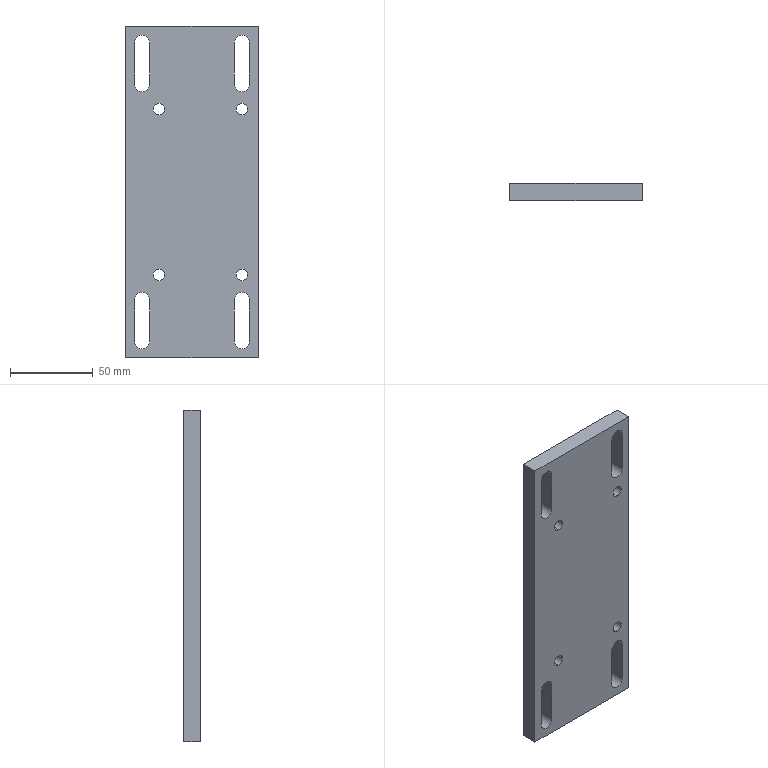Part | STEP file | X77-07007 | 1 solid | 30 faces | box 80 x 10 x 200 mm | volume 147003 mm3 | cylinder 16 | plane 14 | commonest cylinder face diameters 6.8 x8 9 x8
STEP:
#1=CARTESIAN_POINT('',(-304.189,-3.891,153.4));
#2=VERTEX_POINT('',#1);
#3=CARTESIAN_POINT('',(-304.189,-3.891,146.6));
#4=VERTEX_POINT('',#3);
#5=CARTESIAN_POINT('',(-304.189,-3.891,150.));
#6=DIRECTION('',(0.,-1.,0.));
#7=DIRECTION('',(1.,0.,0.));
#8=AXIS2_PLACEMENT_3D('',#5,#6,#7);
#9=CIRCLE('',#8,3.4);
#10=EDGE_CURVE('',#2,#4,#9,.T.);
#11=ORIENTED_EDGE('',*,*,#10,.F.);
#12=CARTESIAN_POINT('',(-304.189,-13.891,153.4));
#13=VERTEX_POINT('',#12);
#14=CARTESIAN_POINT('',(-304.189,-13.891,153.4));
#15=DIRECTION('',(0.,-1.,0.));
#16=VECTOR('',#15,1000.);
#17=LINE('',#14,#16);
#18=EDGE_CURVE('',#2,#13,#17,.T.);
#19=ORIENTED_EDGE('',*,*,#18,.T.);
#20=CARTESIAN_POINT('',(-304.189,-13.891,146.6));
#21=VERTEX_POINT('',#20);
#22=CARTESIAN_POINT('',(-304.189,-13.891,150.));
#23=DIRECTION('',(0.,-1.,0.));
#24=DIRECTION('',(0.,0.,-1.));
#25=AXIS2_PLACEMENT_3D('',#22,#23,#24);
#26=CIRCLE('',#25,3.4);
#27=EDGE_CURVE('',#13,#21,#26,.T.);
#28=ORIENTED_EDGE('',*,*,#27,.T.);
#29=CARTESIAN_POINT('',(-304.189,-13.891,146.6));
#30=DIRECTION('',(0.,-1.,0.));
#31=VECTOR('',#30,1000.);
#32=LINE('',#29,#31);
#33=EDGE_CURVE('',#4,#21,#32,.T.);
#34=ORIENTED_EDGE('',*,*,#33,.F.);
#35=EDGE_LOOP('',(#11,#19,#28,#34));
#36=FACE_OUTER_BOUND('',#35,.T.);
#37=CARTESIAN_POINT('',(-304.189,-13.891,150.));
#38=DIRECTION('',(0.,-1.,0.));
#39=DIRECTION('',(0.,0.,-1.));
#40=AXIS2_PLACEMENT_3D('',#37,#38,#39);
#41=CYLINDRICAL_SURFACE('',#40,3.4);
#42=ADVANCED_FACE('',(#36),#41,.F.);
#43=CARTESIAN_POINT('',(-304.189,-3.891,53.4));
#44=VERTEX_POINT('',#43);
#45=CARTESIAN_POINT('',(-304.189,-3.891,46.6));
#46=VERTEX_POINT('',#45);
#47=CARTESIAN_POINT('',(-304.189,-3.891,50.));
#48=DIRECTION('',(0.,-1.,0.));
#49=DIRECTION('',(1.,0.,0.));
#50=AXIS2_PLACEMENT_3D('',#47,#48,#49);
#51=CIRCLE('',#50,3.4);
#52=EDGE_CURVE('',#44,#46,#51,.T.);
#53=ORIENTED_EDGE('',*,*,#52,.F.);
#54=CARTESIAN_POINT('',(-304.189,-13.891,53.4));
#55=VERTEX_POINT('',#54);
#56=CARTESIAN_POINT('',(-304.189,-13.891,53.4));
#57=DIRECTION('',(0.,-1.,0.));
#58=VECTOR('',#57,1000.);
#59=LINE('',#56,#58);
#60=EDGE_CURVE('',#44,#55,#59,.T.);
#61=ORIENTED_EDGE('',*,*,#60,.T.);
#62=CARTESIAN_POINT('',(-304.189,-13.891,46.6));
#63=VERTEX_POINT('',#62);
#64=CARTESIAN_POINT('',(-304.189,-13.891,50.));
#65=DIRECTION('',(0.,-1.,0.));
#66=DIRECTION('',(0.,0.,-1.));
#67=AXIS2_PLACEMENT_3D('',#64,#65,#66);
#68=CIRCLE('',#67,3.4);
#69=EDGE_CURVE('',#55,#63,#68,.T.);
#70=ORIENTED_EDGE('',*,*,#69,.T.);
#71=CARTESIAN_POINT('',(-304.189,-13.891,46.6));
#72=DIRECTION('',(0.,-1.,0.));
#73=VECTOR('',#72,1000.);
#74=LINE('',#71,#73);
#75=EDGE_CURVE('',#46,#63,#74,.T.);
#76=ORIENTED_EDGE('',*,*,#75,.F.);
#77=EDGE_LOOP('',(#53,#61,#70,#76));
#78=FACE_OUTER_BOUND('',#77,.T.);
#79=CARTESIAN_POINT('',(-304.189,-13.891,50.));
#80=DIRECTION('',(0.,-1.,0.));
#81=DIRECTION('',(0.,0.,-1.));
#82=AXIS2_PLACEMENT_3D('',#79,#80,#81);
#83=CYLINDRICAL_SURFACE('',#82,3.4);
#84=ADVANCED_FACE('',(#78),#83,.F.);
#85=CARTESIAN_POINT('',(-354.189,-3.891,53.4));
#86=VERTEX_POINT('',#85);
#87=CARTESIAN_POINT('',(-354.189,-3.891,46.6));
#88=VERTEX_POINT('',#87);
#89=CARTESIAN_POINT('',(-354.189,-3.891,50.));
#90=DIRECTION('',(0.,-1.,0.));
#91=DIRECTION('',(1.,0.,0.));
#92=AXIS2_PLACEMENT_3D('',#89,#90,#91);
#93=CIRCLE('',#92,3.4);
#94=EDGE_CURVE('',#86,#88,#93,.T.);
#95=ORIENTED_EDGE('',*,*,#94,.F.);
#96=CARTESIAN_POINT('',(-354.189,-13.891,53.4));
#97=VERTEX_POINT('',#96);
#98=CARTESIAN_POINT('',(-354.189,-13.891,53.4));
#99=DIRECTION('',(0.,-1.,0.));
#100=VECTOR('',#99,1000.);
#101=LINE('',#98,#100);
#102=EDGE_CURVE('',#86,#97,#101,.T.);
#103=ORIENTED_EDGE('',*,*,#102,.T.);
#104=CARTESIAN_POINT('',(-354.189,-13.891,46.6));
#105=VERTEX_POINT('',#104);
#106=CARTESIAN_POINT('',(-354.189,-13.891,50.));
#107=DIRECTION('',(0.,-1.,0.));
#108=DIRECTION('',(0.,0.,-1.));
#109=AXIS2_PLACEMENT_3D('',#106,#107,#108);
#110=CIRCLE('',#109,3.4);
#111=EDGE_CURVE('',#97,#105,#110,.T.);
#112=ORIENTED_EDGE('',*,*,#111,.T.);
#113=CARTESIAN_POINT('',(-354.189,-13.891,46.6));
#114=DIRECTION('',(0.,-1.,0.));
#115=VECTOR('',#114,1000.);
#116=LINE('',#113,#115);
#117=EDGE_CURVE('',#88,#105,#116,.T.);
#118=ORIENTED_EDGE('',*,*,#117,.F.);
#119=EDGE_LOOP('',(#95,#103,#112,#118));
#120=FACE_OUTER_BOUND('',#119,.T.);
#121=CARTESIAN_POINT('',(-354.189,-13.891,50.));
#122=DIRECTION('',(0.,-1.,0.));
#123=DIRECTION('',(0.,0.,-1.));
#124=AXIS2_PLACEMENT_3D('',#121,#122,#123);
#125=CYLINDRICAL_SURFACE('',#124,3.4);
#126=ADVANCED_FACE('',(#120),#125,.F.);
#127=CARTESIAN_POINT('',(-354.189,-3.891,153.4));
#128=VERTEX_POINT('',#127);
#129=CARTESIAN_POINT('',(-354.189,-3.891,146.6));
#130=VERTEX_POINT('',#129);
#131=CARTESIAN_POINT('',(-354.189,-3.891,150.));
#132=DIRECTION('',(0.,-1.,0.));
#133=DIRECTION('',(1.,0.,0.));
#134=AXIS2_PLACEMENT_3D('',#131,#132,#133);
#135=CIRCLE('',#134,3.4);
#136=EDGE_CURVE('',#128,#130,#135,.T.);
#137=ORIENTED_EDGE('',*,*,#136,.F.);
#138=CARTESIAN_POINT('',(-354.189,-13.891,153.4));
#139=VERTEX_POINT('',#138);
#140=CARTESIAN_POINT('',(-354.189,-13.891,153.4));
#141=DIRECTION('',(0.,-1.,0.));
#142=VECTOR('',#141,1000.);
#143=LINE('',#140,#142);
#144=EDGE_CURVE('',#128,#139,#143,.T.);
#145=ORIENTED_EDGE('',*,*,#144,.T.);
#146=CARTESIAN_POINT('',(-354.189,-13.891,146.6));
#147=VERTEX_POINT('',#146);
#148=CARTESIAN_POINT('',(-354.189,-13.891,150.));
#149=DIRECTION('',(0.,-1.,0.));
#150=DIRECTION('',(0.,0.,-1.));
#151=AXIS2_PLACEMENT_3D('',#148,#149,#150);
#152=CIRCLE('',#151,3.4);
#153=EDGE_CURVE('',#139,#147,#152,.T.);
#154=ORIENTED_EDGE('',*,*,#153,.T.);
#155=CARTESIAN_POINT('',(-354.189,-13.891,146.6));
#156=DIRECTION('',(0.,-1.,0.));
#157=VECTOR('',#156,1000.);
#158=LINE('',#155,#157);
#159=EDGE_CURVE('',#130,#147,#158,.T.);
#160=ORIENTED_EDGE('',*,*,#159,.F.);
#161=EDGE_LOOP('',(#137,#145,#154,#160));
#162=FACE_OUTER_BOUND('',#161,.T.);
#163=CARTESIAN_POINT('',(-354.189,-13.891,150.));
#164=DIRECTION('',(0.,-1.,0.));
#165=DIRECTION('',(0.,0.,-1.));
#166=AXIS2_PLACEMENT_3D('',#163,#164,#165);
#167=CYLINDRICAL_SURFACE('',#166,3.4);
#168=ADVANCED_FACE('',(#162),#167,.F.);
#169=CARTESIAN_POINT('',(-294.189,-13.891,0.));
#170=VERTEX_POINT('',#169);
#171=CARTESIAN_POINT('',(-294.189,-3.891,0.));
#172=VERTEX_POINT('',#171);
#173=CARTESIAN_POINT('',(-294.189,-13.891,0.));
#174=DIRECTION('',(0.,1.,0.));
#175=VECTOR('',#174,1000.);
#176=LINE('',#173,#175);
#177=EDGE_CURVE('',#170,#172,#176,.T.);
#178=ORIENTED_EDGE('',*,*,#177,.T.);
#179=CARTESIAN_POINT('',(-294.189,-3.891,200.));
#180=VERTEX_POINT('',#179);
#181=CARTESIAN_POINT('',(-294.189,-3.891,200.));
#182=DIRECTION('',(0.,0.,-1.));
#183=VECTOR('',#182,1000.);
#184=LINE('',#181,#183);
#185=EDGE_CURVE('',#180,#172,#184,.T.);
#186=ORIENTED_EDGE('',*,*,#185,.F.);
#187=CARTESIAN_POINT('',(-294.189,-13.891,200.));
#188=VERTEX_POINT('',#187);
#189=CARTESIAN_POINT('',(-294.189,-13.891,200.));
#190=DIRECTION('',(0.,1.,0.));
#191=VECTOR('',#190,1000.);
#192=LINE('',#189,#191);
#193=EDGE_CURVE('',#188,#180,#192,.T.);
#194=ORIENTED_EDGE('',*,*,#193,.F.);
#195=CARTESIAN_POINT('',(-294.189,-13.891,200.));
#196=DIRECTION('',(0.,0.,-1.));
#197=VECTOR('',#196,1000.);
#198=LINE('',#195,#197);
#199=EDGE_CURVE('',#188,#170,#198,.T.);
#200=ORIENTED_EDGE('',*,*,#199,.T.);
#201=EDGE_LOOP('',(#178,#186,#194,#200));
#202=FACE_OUTER_BOUND('',#201,.T.);
#203=CARTESIAN_POINT('',(-294.189,-13.891,200.));
#204=DIRECTION('',(-1.,0.,0.));
#205=DIRECTION('',(0.,0.,1.));
#206=AXIS2_PLACEMENT_3D('',#203,#204,#205);
#207=PLANE('',#206);
#208=ADVANCED_FACE('',(#202),#207,.F.);
#209=CARTESIAN_POINT('',(-368.689,-3.891,35.));
#210=VERTEX_POINT('',#209);
#211=CARTESIAN_POINT('',(-368.689,-3.891,10.));
#212=VERTEX_POINT('',#211);
#213=CARTESIAN_POINT('',(-368.689,-3.891,200.));
#214=DIRECTION('',(0.,0.,-1.));
#215=VECTOR('',#214,1000.);
#216=LINE('',#213,#215);
#217=EDGE_CURVE('',#210,#212,#216,.T.);
#218=ORIENTED_EDGE('',*,*,#217,.T.);
#219=CARTESIAN_POINT('',(-359.689,-3.891,10.));
#220=VERTEX_POINT('',#219);
#221=CARTESIAN_POINT('',(-364.189,-3.891,10.));
#222=DIRECTION('',(0.,-1.,0.));
#223=DIRECTION('',(1.,0.,0.));
#224=AXIS2_PLACEMENT_3D('',#221,#222,#223);
#225=CIRCLE('',#224,4.5);
#226=EDGE_CURVE('',#212,#220,#225,.T.);
#227=ORIENTED_EDGE('',*,*,#226,.T.);
#228=CARTESIAN_POINT('',(-359.689,-3.891,35.));
#229=VERTEX_POINT('',#228);
#230=CARTESIAN_POINT('',(-359.689,-3.891,200.));
#231=DIRECTION('',(0.,0.,1.));
#232=VECTOR('',#231,1000.);
#233=LINE('',#230,#232);
#234=EDGE_CURVE('',#220,#229,#233,.T.);
#235=ORIENTED_EDGE('',*,*,#234,.T.);
#236=CARTESIAN_POINT('',(-364.189,-3.891,35.));
#237=DIRECTION('',(0.,-1.,0.));
#238=DIRECTION('',(1.,0.,0.));
#239=AXIS2_PLACEMENT_3D('',#236,#237,#238);
#240=CIRCLE('',#239,4.5);
#241=EDGE_CURVE('',#229,#210,#240,.T.);
#242=ORIENTED_EDGE('',*,*,#241,.T.);
#243=EDGE_LOOP('',(#218,#227,#235,#242));
#244=FACE_BOUND('',#243,.T.);
#245=CARTESIAN_POINT('',(-359.689,-3.891,165.));
#246=VERTEX_POINT('',#245);
#247=CARTESIAN_POINT('',(-359.689,-3.891,190.));
#248=VERTEX_POINT('',#247);
#249=CARTESIAN_POINT('',(-359.689,-3.891,200.));
#250=DIRECTION('',(0.,0.,1.));
#251=VECTOR('',#250,1000.);
#252=LINE('',#249,#251);
#253=EDGE_CURVE('',#246,#248,#252,.T.);
#254=ORIENTED_EDGE('',*,*,#253,.T.);
#255=CARTESIAN_POINT('',(-368.689,-3.891,190.));
#256=VERTEX_POINT('',#255);
#257=CARTESIAN_POINT('',(-364.189,-3.891,190.));
#258=DIRECTION('',(0.,-1.,0.));
#259=DIRECTION('',(1.,0.,0.));
#260=AXIS2_PLACEMENT_3D('',#257,#258,#259);
#261=CIRCLE('',#260,4.5);
#262=EDGE_CURVE('',#248,#256,#261,.T.);
#263=ORIENTED_EDGE('',*,*,#262,.T.);
#264=CARTESIAN_POINT('',(-368.689,-3.891,165.));
#265=VERTEX_POINT('',#264);
#266=CARTESIAN_POINT('',(-368.689,-3.891,200.));
#267=DIRECTION('',(0.,0.,-1.));
#268=VECTOR('',#267,1000.);
#269=LINE('',#266,#268);
#270=EDGE_CURVE('',#256,#265,#269,.T.);
#271=ORIENTED_EDGE('',*,*,#270,.T.);
#272=CARTESIAN_POINT('',(-364.189,-3.891,165.));
#273=DIRECTION('',(0.,-1.,0.));
#274=DIRECTION('',(1.,0.,0.));
#275=AXIS2_PLACEMENT_3D('',#272,#273,#274);
#276=CIRCLE('',#275,4.5);
#277=EDGE_CURVE('',#265,#246,#276,.T.);
#278=ORIENTED_EDGE('',*,*,#277,.T.);
#279=EDGE_LOOP('',(#254,#263,#271,#278));
#280=FACE_BOUND('',#279,.T.);
#281=CARTESIAN_POINT('',(-308.689,-3.891,35.));
#282=VERTEX_POINT('',#281);
#283=CARTESIAN_POINT('',(-308.689,-3.891,10.));
#284=VERTEX_POINT('',#283);
#285=CARTESIAN_POINT('',(-308.689,-3.891,200.));
#286=DIRECTION('',(0.,0.,-1.));
#287=VECTOR('',#286,1000.);
#288=LINE('',#285,#287);
#289=EDGE_CURVE('',#282,#284,#288,.T.);
#290=ORIENTED_EDGE('',*,*,#289,.T.);
#291=CARTESIAN_POINT('',(-299.689,-3.891,10.));
#292=VERTEX_POINT('',#291);
#293=CARTESIAN_POINT('',(-304.189,-3.891,10.));
#294=DIRECTION('',(0.,-1.,0.));
#295=DIRECTION('',(1.,0.,0.));
#296=AXIS2_PLACEMENT_3D('',#293,#294,#295);
#297=CIRCLE('',#296,4.5);
#298=EDGE_CURVE('',#284,#292,#297,.T.);
#299=ORIENTED_EDGE('',*,*,#298,.T.);
#300=CARTESIAN_POINT('',(-299.689,-3.891,35.));
#301=VERTEX_POINT('',#300);
#302=CARTESIAN_POINT('',(-299.689,-3.891,200.));
#303=DIRECTION('',(0.,0.,1.));
#304=VECTOR('',#303,1000.);
#305=LINE('',#302,#304);
#306=EDGE_CURVE('',#292,#301,#305,.T.);
#307=ORIENTED_EDGE('',*,*,#306,.T.);
#308=CARTESIAN_POINT('',(-304.189,-3.891,35.));
#309=DIRECTION('',(0.,-1.,0.));
#310=DIRECTION('',(1.,0.,0.));
#311=AXIS2_PLACEMENT_3D('',#308,#309,#310);
#312=CIRCLE('',#311,4.5);
#313=EDGE_CURVE('',#301,#282,#312,.T.);
#314=ORIENTED_EDGE('',*,*,#313,.T.);
#315=EDGE_LOOP('',(#290,#299,#307,#314));
#316=FACE_BOUND('',#315,.T.);
#317=CARTESIAN_POINT('',(-299.689,-3.891,165.));
#318=VERTEX_POINT('',#317);
#319=CARTESIAN_POINT('',(-299.689,-3.891,190.));
#320=VERTEX_POINT('',#319);
#321=CARTESIAN_POINT('',(-299.689,-3.891,200.));
#322=DIRECTION('',(0.,0.,1.));
#323=VECTOR('',#322,1000.);
#324=LINE('',#321,#323);
#325=EDGE_CURVE('',#318,#320,#324,.T.);
#326=ORIENTED_EDGE('',*,*,#325,.T.);
#327=CARTESIAN_POINT('',(-308.689,-3.891,190.));
#328=VERTEX_POINT('',#327);
#329=CARTESIAN_POINT('',(-304.189,-3.891,190.));
#330=DIRECTION('',(0.,-1.,0.));
#331=DIRECTION('',(1.,0.,0.));
#332=AXIS2_PLACEMENT_3D('',#329,#330,#331);
#333=CIRCLE('',#332,4.5);
#334=EDGE_CURVE('',#320,#328,#333,.T.);
#335=ORIENTED_EDGE('',*,*,#334,.T.);
#336=CARTESIAN_POINT('',(-308.689,-3.891,165.));
#337=VERTEX_POINT('',#336);
#338=CARTESIAN_POINT('',(-308.689,-3.891,200.));
#339=DIRECTION('',(0.,0.,-1.));
#340=VECTOR('',#339,1000.);
#341=LINE('',#338,#340);
#342=EDGE_CURVE('',#328,#337,#341,.T.);
#343=ORIENTED_EDGE('',*,*,#342,.T.);
#344=CARTESIAN_POINT('',(-304.189,-3.891,165.));
#345=DIRECTION('',(0.,-1.,0.));
#346=DIRECTION('',(1.,0.,0.));
#347=AXIS2_PLACEMENT_3D('',#344,#345,#346);
#348=CIRCLE('',#347,4.5);
#349=EDGE_CURVE('',#337,#318,#348,.T.);
#350=ORIENTED_EDGE('',*,*,#349,.T.);
#351=EDGE_LOOP('',(#326,#335,#343,#350));
#352=FACE_BOUND('',#351,.T.);
#353=CARTESIAN_POINT('',(-304.189,-3.891,150.));
#354=DIRECTION('',(0.,-1.,0.));
#355=DIRECTION('',(1.,0.,0.));
#356=AXIS2_PLACEMENT_3D('',#353,#354,#355);
#357=CIRCLE('',#356,3.4);
#358=EDGE_CURVE('',#4,#2,#357,.T.);
#359=ORIENTED_EDGE('',*,*,#358,.T.);
#360=ORIENTED_EDGE('',*,*,#10,.T.);
#361=EDGE_LOOP('',(#359,#360));
#362=FACE_BOUND('',#361,.T.);
#363=CARTESIAN_POINT('',(-304.189,-3.891,50.));
#364=DIRECTION('',(0.,-1.,0.));
#365=DIRECTION('',(1.,0.,0.));
#366=AXIS2_PLACEMENT_3D('',#363,#364,#365);
#367=CIRCLE('',#366,3.4);
#368=EDGE_CURVE('',#46,#44,#367,.T.);
#369=ORIENTED_EDGE('',*,*,#368,.T.);
#370=ORIENTED_EDGE('',*,*,#52,.T.);
#371=EDGE_LOOP('',(#369,#370));
#372=FACE_BOUND('',#371,.T.);
#373=CARTESIAN_POINT('',(-354.189,-3.891,50.));
#374=DIRECTION('',(0.,-1.,0.));
#375=DIRECTION('',(1.,0.,0.));
#376=AXIS2_PLACEMENT_3D('',#373,#374,#375);
#377=CIRCLE('',#376,3.4);
#378=EDGE_CURVE('',#88,#86,#377,.T.);
#379=ORIENTED_EDGE('',*,*,#378,.T.);
#380=ORIENTED_EDGE('',*,*,#94,.T.);
#381=EDGE_LOOP('',(#379,#380));
#382=FACE_BOUND('',#381,.T.);
#383=CARTESIAN_POINT('',(-354.189,-3.891,150.));
#384=DIRECTION('',(0.,-1.,0.));
#385=DIRECTION('',(1.,0.,0.));
#386=AXIS2_PLACEMENT_3D('',#383,#384,#385);
#387=CIRCLE('',#386,3.4);
#388=EDGE_CURVE('',#130,#128,#387,.T.);
#389=ORIENTED_EDGE('',*,*,#388,.T.);
#390=ORIENTED_EDGE('',*,*,#136,.T.);
#391=EDGE_LOOP('',(#389,#390));
#392=FACE_BOUND('',#391,.T.);
#393=CARTESIAN_POINT('',(-374.189,-3.891,0.));
#394=VERTEX_POINT('',#393);
#395=CARTESIAN_POINT('',(-294.189,-3.891,0.));
#396=DIRECTION('',(-1.,0.,0.));
#397=VECTOR('',#396,1000.);
#398=LINE('',#395,#397);
#399=EDGE_CURVE('',#172,#394,#398,.T.);
#400=ORIENTED_EDGE('',*,*,#399,.T.);
#401=CARTESIAN_POINT('',(-374.189,-3.891,200.));
#402=VERTEX_POINT('',#401);
#403=CARTESIAN_POINT('',(-374.189,-3.891,200.));
#404=DIRECTION('',(0.,0.,-1.));
#405=VECTOR('',#404,1000.);
#406=LINE('',#403,#405);
#407=EDGE_CURVE('',#402,#394,#406,.T.);
#408=ORIENTED_EDGE('',*,*,#407,.F.);
#409=CARTESIAN_POINT('',(-294.189,-3.891,200.));
#410=DIRECTION('',(-1.,0.,0.));
#411=VECTOR('',#410,1000.);
#412=LINE('',#409,#411);
#413=EDGE_CURVE('',#180,#402,#412,.T.);
#414=ORIENTED_EDGE('',*,*,#413,.F.);
#415=ORIENTED_EDGE('',*,*,#185,.T.);
#416=EDGE_LOOP('',(#400,#408,#414,#415));
#417=FACE_OUTER_BOUND('',#416,.T.);
#418=CARTESIAN_POINT('',(-294.189,-3.891,200.));
#419=DIRECTION('',(0.,-1.,0.));
#420=DIRECTION('',(1.,0.,0.));
#421=AXIS2_PLACEMENT_3D('',#418,#419,#420);
#422=PLANE('',#421);
#423=ADVANCED_FACE('',(#244,#280,#316,#352,#362,#372,#382,#392,#417),#422,.F.);
#424=CARTESIAN_POINT('',(-374.189,-13.891,0.));
#425=VERTEX_POINT('',#424);
#426=CARTESIAN_POINT('',(-374.189,-13.891,0.));
#427=DIRECTION('',(0.,-1.,0.));
#428=VECTOR('',#427,1000.);
#429=LINE('',#426,#428);
#430=EDGE_CURVE('',#394,#425,#429,.T.);
#431=ORIENTED_EDGE('',*,*,#430,.T.);
#432=CARTESIAN_POINT('',(-374.189,-13.891,200.));
#433=VERTEX_POINT('',#432);
#434=CARTESIAN_POINT('',(-374.189,-13.891,200.));
#435=DIRECTION('',(0.,0.,-1.));
#436=VECTOR('',#435,1000.);
#437=LINE('',#434,#436);
#438=EDGE_CURVE('',#433,#425,#437,.T.);
#439=ORIENTED_EDGE('',*,*,#438,.F.);
#440=CARTESIAN_POINT('',(-374.189,-13.891,200.));
#441=DIRECTION('',(0.,-1.,0.));
#442=VECTOR('',#441,1000.);
#443=LINE('',#440,#442);
#444=EDGE_CURVE('',#402,#433,#443,.T.);
#445=ORIENTED_EDGE('',*,*,#444,.F.);
#446=ORIENTED_EDGE('',*,*,#407,.T.);
#447=EDGE_LOOP('',(#431,#439,#445,#446));
#448=FACE_OUTER_BOUND('',#447,.T.);
#449=CARTESIAN_POINT('',(-374.189,-13.891,200.));
#450=DIRECTION('',(1.,0.,0.));
#451=DIRECTION('',(0.,0.,-1.));
#452=AXIS2_PLACEMENT_3D('',#449,#450,#451);
#453=PLANE('',#452);
#454=ADVANCED_FACE('',(#448),#453,.F.);
#455=CARTESIAN_POINT('',(-359.689,-13.891,10.));
#456=VERTEX_POINT('',#455);
#457=CARTESIAN_POINT('',(-359.689,-13.891,35.));
#458=VERTEX_POINT('',#457);
#459=CARTESIAN_POINT('',(-359.689,-13.891,10.));
#460=DIRECTION('',(0.,0.,1.));
#461=VECTOR('',#460,1000.);
#462=LINE('',#459,#461);
#463=EDGE_CURVE('',#456,#458,#462,.T.);
#464=ORIENTED_EDGE('',*,*,#463,.F.);
#465=CARTESIAN_POINT('',(-368.689,-13.891,10.));
#466=VERTEX_POINT('',#465);
#467=CARTESIAN_POINT('',(-364.189,-13.891,10.));
#468=DIRECTION('',(0.,-1.,0.));
#469=DIRECTION('',(1.,0.,0.));
#470=AXIS2_PLACEMENT_3D('',#467,#468,#469);
#471=CIRCLE('',#470,4.5);
#472=EDGE_CURVE('',#466,#456,#471,.T.);
#473=ORIENTED_EDGE('',*,*,#472,.F.);
#474=CARTESIAN_POINT('',(-368.689,-13.891,35.));
#475=VERTEX_POINT('',#474);
#476=CARTESIAN_POINT('',(-368.689,-13.891,10.));
#477=DIRECTION('',(0.,0.,-1.));
#478=VECTOR('',#477,1000.);
#479=LINE('',#476,#478);
#480=EDGE_CURVE('',#475,#466,#479,.T.);
#481=ORIENTED_EDGE('',*,*,#480,.F.);
#482=CARTESIAN_POINT('',(-364.189,-13.891,35.));
#483=DIRECTION('',(0.,-1.,0.));
#484=DIRECTION('',(1.,0.,0.));
#485=AXIS2_PLACEMENT_3D('',#482,#483,#484);
#486=CIRCLE('',#485,4.5);
#487=EDGE_CURVE('',#458,#475,#486,.T.);
#488=ORIENTED_EDGE('',*,*,#487,.F.);
#489=EDGE_LOOP('',(#464,#473,#481,#488));
#490=FACE_BOUND('',#489,.T.);
#491=CARTESIAN_POINT('',(-368.689,-13.891,190.));
#492=VERTEX_POINT('',#491);
#493=CARTESIAN_POINT('',(-368.689,-13.891,165.));
#494=VERTEX_POINT('',#493);
#495=CARTESIAN_POINT('',(-368.689,-13.891,190.));
#496=DIRECTION('',(0.,0.,-1.));
#497=VECTOR('',#496,1000.);
#498=LINE('',#495,#497);
#499=EDGE_CURVE('',#492,#494,#498,.T.);
#500=ORIENTED_EDGE('',*,*,#499,.F.);
#501=CARTESIAN_POINT('',(-359.689,-13.891,190.));
#502=VERTEX_POINT('',#501);
#503=CARTESIAN_POINT('',(-364.189,-13.891,190.));
#504=DIRECTION('',(0.,-1.,0.));
#505=DIRECTION('',(-1.,0.,0.));
#506=AXIS2_PLACEMENT_3D('',#503,#504,#505);
#507=CIRCLE('',#506,4.5);
#508=EDGE_CURVE('',#502,#492,#507,.T.);
#509=ORIENTED_EDGE('',*,*,#508,.F.);
#510=CARTESIAN_POINT('',(-359.689,-13.891,165.));
#511=VERTEX_POINT('',#510);
#512=CARTESIAN_POINT('',(-359.689,-13.891,190.));
#513=DIRECTION('',(0.,0.,1.));
#514=VECTOR('',#513,1000.);
#515=LINE('',#512,#514);
#516=EDGE_CURVE('',#511,#502,#515,.T.);
#517=ORIENTED_EDGE('',*,*,#516,.F.);
#518=CARTESIAN_POINT('',(-364.189,-13.891,165.));
#519=DIRECTION('',(0.,-1.,0.));
#520=DIRECTION('',(-1.,0.,0.));
#521=AXIS2_PLACEMENT_3D('',#518,#519,#520);
#522=CIRCLE('',#521,4.5);
#523=EDGE_CURVE('',#494,#511,#522,.T.);
#524=ORIENTED_EDGE('',*,*,#523,.F.);
#525=EDGE_LOOP('',(#500,#509,#517,#524));
#526=FACE_BOUND('',#525,.T.);
#527=CARTESIAN_POINT('',(-299.689,-13.891,10.));
#528=VERTEX_POINT('',#527);
#529=CARTESIAN_POINT('',(-299.689,-13.891,35.));
#530=VERTEX_POINT('',#529);
#531=CARTESIAN_POINT('',(-299.689,-13.891,10.));
#532=DIRECTION('',(0.,0.,1.));
#533=VECTOR('',#532,1000.);
#534=LINE('',#531,#533);
#535=EDGE_CURVE('',#528,#530,#534,.T.);
#536=ORIENTED_EDGE('',*,*,#535,.F.);
#537=CARTESIAN_POINT('',(-308.689,-13.891,10.));
#538=VERTEX_POINT('',#537);
#539=CARTESIAN_POINT('',(-304.189,-13.891,10.));
#540=DIRECTION('',(0.,-1.,0.));
#541=DIRECTION('',(-1.,0.,0.));
#542=AXIS2_PLACEMENT_3D('',#539,#540,#541);
#543=CIRCLE('',#542,4.5);
#544=EDGE_CURVE('',#538,#528,#543,.T.);
#545=ORIENTED_EDGE('',*,*,#544,.F.);
#546=CARTESIAN_POINT('',(-308.689,-13.891,35.));
#547=VERTEX_POINT('',#546);
#548=CARTESIAN_POINT('',(-308.689,-13.891,10.));
#549=DIRECTION('',(0.,0.,-1.));
#550=VECTOR('',#549,1000.);
#551=LINE('',#548,#550);
#552=EDGE_CURVE('',#547,#538,#551,.T.);
#553=ORIENTED_EDGE('',*,*,#552,.F.);
#554=CARTESIAN_POINT('',(-304.189,-13.891,35.));
#555=DIRECTION('',(0.,-1.,0.));
#556=DIRECTION('',(-1.,0.,0.));
#557=AXIS2_PLACEMENT_3D('',#554,#555,#556);
#558=CIRCLE('',#557,4.5);
#559=EDGE_CURVE('',#530,#547,#558,.T.);
#560=ORIENTED_EDGE('',*,*,#559,.F.);
#561=EDGE_LOOP('',(#536,#545,#553,#560));
#562=FACE_BOUND('',#561,.T.);
#563=CARTESIAN_POINT('',(-308.689,-13.891,190.));
#564=VERTEX_POINT('',#563);
#565=CARTESIAN_POINT('',(-308.689,-13.891,165.));
#566=VERTEX_POINT('',#565);
#567=CARTESIAN_POINT('',(-308.689,-13.891,190.));
#568=DIRECTION('',(0.,0.,-1.));
#569=VECTOR('',#568,1000.);
#570=LINE('',#567,#569);
#571=EDGE_CURVE('',#564,#566,#570,.T.);
#572=ORIENTED_EDGE('',*,*,#571,.F.);
#573=CARTESIAN_POINT('',(-299.689,-13.891,190.));
#574=VERTEX_POINT('',#573);
#575=CARTESIAN_POINT('',(-304.189,-13.891,190.));
#576=DIRECTION('',(0.,-1.,0.));
#577=DIRECTION('',(1.,0.,0.));
#578=AXIS2_PLACEMENT_3D('',#575,#576,#577);
#579=CIRCLE('',#578,4.5);
#580=EDGE_CURVE('',#574,#564,#579,.T.);
#581=ORIENTED_EDGE('',*,*,#580,.F.);
#582=CARTESIAN_POINT('',(-299.689,-13.891,165.));
#583=VERTEX_POINT('',#582);
#584=CARTESIAN_POINT('',(-299.689,-13.891,190.));
#585=DIRECTION('',(0.,0.,1.));
#586=VECTOR('',#585,1000.);
#587=LINE('',#584,#586);
#588=EDGE_CURVE('',#583,#574,#587,.T.);
#589=ORIENTED_EDGE('',*,*,#588,.F.);
#590=CARTESIAN_POINT('',(-304.189,-13.891,165.));
#591=DIRECTION('',(0.,-1.,0.));
#592=DIRECTION('',(1.,0.,0.));
#593=AXIS2_PLACEMENT_3D('',#590,#591,#592);
#594=CIRCLE('',#593,4.5);
#595=EDGE_CURVE('',#566,#583,#594,.T.);
#596=ORIENTED_EDGE('',*,*,#595,.F.);
#597=EDGE_LOOP('',(#572,#581,#589,#596));
#598=FACE_BOUND('',#597,.T.);
#599=CARTESIAN_POINT('',(-304.189,-13.891,150.));
#600=DIRECTION('',(0.,-1.,0.));
#601=DIRECTION('',(0.,0.,-1.));
#602=AXIS2_PLACEMENT_3D('',#599,#600,#601);
#603=CIRCLE('',#602,3.4);
#604=EDGE_CURVE('',#21,#13,#603,.T.);
#605=ORIENTED_EDGE('',*,*,#604,.F.);
#606=ORIENTED_EDGE('',*,*,#27,.F.);
#607=EDGE_LOOP('',(#605,#606));
#608=FACE_BOUND('',#607,.T.);
#609=CARTESIAN_POINT('',(-304.189,-13.891,50.));
#610=DIRECTION('',(0.,-1.,0.));
#611=DIRECTION('',(0.,0.,-1.));
#612=AXIS2_PLACEMENT_3D('',#609,#610,#611);
#613=CIRCLE('',#612,3.4);
#614=EDGE_CURVE('',#63,#55,#613,.T.);
#615=ORIENTED_EDGE('',*,*,#614,.F.);
#616=ORIENTED_EDGE('',*,*,#69,.F.);
#617=EDGE_LOOP('',(#615,#616));
#618=FACE_BOUND('',#617,.T.);
#619=CARTESIAN_POINT('',(-354.189,-13.891,50.));
#620=DIRECTION('',(0.,-1.,0.));
#621=DIRECTION('',(0.,0.,-1.));
#622=AXIS2_PLACEMENT_3D('',#619,#620,#621);
#623=CIRCLE('',#622,3.4);
#624=EDGE_CURVE('',#105,#97,#623,.T.);
#625=ORIENTED_EDGE('',*,*,#624,.F.);
#626=ORIENTED_EDGE('',*,*,#111,.F.);
#627=EDGE_LOOP('',(#625,#626));
#628=FACE_BOUND('',#627,.T.);
#629=CARTESIAN_POINT('',(-354.189,-13.891,150.));
#630=DIRECTION('',(0.,-1.,0.));
#631=DIRECTION('',(0.,0.,-1.));
#632=AXIS2_PLACEMENT_3D('',#629,#630,#631);
#633=CIRCLE('',#632,3.4);
#634=EDGE_CURVE('',#147,#139,#633,.T.);
#635=ORIENTED_EDGE('',*,*,#634,.F.);
#636=ORIENTED_EDGE('',*,*,#153,.F.);
#637=EDGE_LOOP('',(#635,#636));
#638=FACE_BOUND('',#637,.T.);
#639=CARTESIAN_POINT('',(-294.189,-13.891,0.));
#640=DIRECTION('',(1.,0.,0.));
#641=VECTOR('',#640,1000.);
#642=LINE('',#639,#641);
#643=EDGE_CURVE('',#425,#170,#642,.T.);
#644=ORIENTED_EDGE('',*,*,#643,.T.);
#645=ORIENTED_EDGE('',*,*,#199,.F.);
#646=CARTESIAN_POINT('',(-294.189,-13.891,200.));
#647=DIRECTION('',(1.,0.,0.));
#648=VECTOR('',#647,1000.);
#649=LINE('',#646,#648);
#650=EDGE_CURVE('',#433,#188,#649,.T.);
#651=ORIENTED_EDGE('',*,*,#650,.F.);
#652=ORIENTED_EDGE('',*,*,#438,.T.);
#653=EDGE_LOOP('',(#644,#645,#651,#652));
#654=FACE_OUTER_BOUND('',#653,.T.);
#655=CARTESIAN_POINT('',(-294.189,-13.891,200.));
#656=DIRECTION('',(0.,1.,0.));
#657=DIRECTION('',(-1.,0.,0.));
#658=AXIS2_PLACEMENT_3D('',#655,#656,#657);
#659=PLANE('',#658);
#660=ADVANCED_FACE('',(#490,#526,#562,#598,#608,#618,#628,#638,#654),#659,.F.);
#661=ORIENTED_EDGE('',*,*,#193,.T.);
#662=ORIENTED_EDGE('',*,*,#413,.T.);
#663=ORIENTED_EDGE('',*,*,#444,.T.);
#664=ORIENTED_EDGE('',*,*,#650,.T.);
#665=EDGE_LOOP('',(#661,#662,#663,#664));
#666=FACE_OUTER_BOUND('',#665,.T.);
#667=CARTESIAN_POINT('',(-294.189,-3.891,200.));
#668=DIRECTION('',(0.,0.,1.));
#669=DIRECTION('',(1.,0.,0.));
#670=AXIS2_PLACEMENT_3D('',#667,#668,#669);
#671=PLANE('',#670);
#672=ADVANCED_FACE('',(#666),#671,.T.);
#673=ORIENTED_EDGE('',*,*,#177,.F.);
#674=ORIENTED_EDGE('',*,*,#643,.F.);
#675=ORIENTED_EDGE('',*,*,#430,.F.);
#676=ORIENTED_EDGE('',*,*,#399,.F.);
#677=EDGE_LOOP('',(#673,#674,#675,#676));
#678=FACE_OUTER_BOUND('',#677,.T.);
#679=CARTESIAN_POINT('',(-294.189,-3.891,0.));
#680=DIRECTION('',(0.,0.,1.));
#681=DIRECTION('',(1.,0.,0.));
#682=AXIS2_PLACEMENT_3D('',#679,#680,#681);
#683=PLANE('',#682);
#684=ADVANCED_FACE('',(#678),#683,.F.);
#685=ORIENTED_EDGE('',*,*,#144,.F.);
#686=ORIENTED_EDGE('',*,*,#388,.F.);
#687=ORIENTED_EDGE('',*,*,#159,.T.);
#688=ORIENTED_EDGE('',*,*,#634,.T.);
#689=EDGE_LOOP('',(#685,#686,#687,#688));
#690=FACE_OUTER_BOUND('',#689,.T.);
#691=CARTESIAN_POINT('',(-354.189,-13.891,150.));
#692=DIRECTION('',(0.,-1.,0.));
#693=DIRECTION('',(0.,0.,-1.));
#694=AXIS2_PLACEMENT_3D('',#691,#692,#693);
#695=CYLINDRICAL_SURFACE('',#694,3.4);
#696=ADVANCED_FACE('',(#690),#695,.F.);
#697=ORIENTED_EDGE('',*,*,#102,.F.);
#698=ORIENTED_EDGE('',*,*,#378,.F.);
#699=ORIENTED_EDGE('',*,*,#117,.T.);
#700=ORIENTED_EDGE('',*,*,#624,.T.);
#701=EDGE_LOOP('',(#697,#698,#699,#700));
#702=FACE_OUTER_BOUND('',#701,.T.);
#703=CARTESIAN_POINT('',(-354.189,-13.891,50.));
#704=DIRECTION('',(0.,-1.,0.));
#705=DIRECTION('',(0.,0.,-1.));
#706=AXIS2_PLACEMENT_3D('',#703,#704,#705);
#707=CYLINDRICAL_SURFACE('',#706,3.4);
#708=ADVANCED_FACE('',(#702),#707,.F.);
#709=ORIENTED_EDGE('',*,*,#60,.F.);
#710=ORIENTED_EDGE('',*,*,#368,.F.);
#711=ORIENTED_EDGE('',*,*,#75,.T.);
#712=ORIENTED_EDGE('',*,*,#614,.T.);
#713=EDGE_LOOP('',(#709,#710,#711,#712));
#714=FACE_OUTER_BOUND('',#713,.T.);
#715=CARTESIAN_POINT('',(-304.189,-13.891,50.));
#716=DIRECTION('',(0.,-1.,0.));
#717=DIRECTION('',(0.,0.,-1.));
#718=AXIS2_PLACEMENT_3D('',#715,#716,#717);
#719=CYLINDRICAL_SURFACE('',#718,3.4);
#720=ADVANCED_FACE('',(#714),#719,.F.);
#721=ORIENTED_EDGE('',*,*,#18,.F.);
#722=ORIENTED_EDGE('',*,*,#358,.F.);
#723=ORIENTED_EDGE('',*,*,#33,.T.);
#724=ORIENTED_EDGE('',*,*,#604,.T.);
#725=EDGE_LOOP('',(#721,#722,#723,#724));
#726=FACE_OUTER_BOUND('',#725,.T.);
#727=CARTESIAN_POINT('',(-304.189,-13.891,150.));
#728=DIRECTION('',(0.,-1.,0.));
#729=DIRECTION('',(0.,0.,-1.));
#730=AXIS2_PLACEMENT_3D('',#727,#728,#729);
#731=CYLINDRICAL_SURFACE('',#730,3.4);
#732=ADVANCED_FACE('',(#726),#731,.F.);
#733=CARTESIAN_POINT('',(-299.689,286.109,190.));
#734=DIRECTION('',(0.,-1.,0.));
#735=VECTOR('',#734,1000.);
#736=LINE('',#733,#735);
#737=EDGE_CURVE('',#320,#574,#736,.T.);
#738=ORIENTED_EDGE('',*,*,#737,.T.);
#739=ORIENTED_EDGE('',*,*,#580,.T.);
#740=CARTESIAN_POINT('',(-308.689,286.109,190.));
#741=DIRECTION('',(0.,-1.,0.));
#742=VECTOR('',#741,1000.);
#743=LINE('',#740,#742);
#744=EDGE_CURVE('',#328,#564,#743,.T.);
#745=ORIENTED_EDGE('',*,*,#744,.F.);
#746=ORIENTED_EDGE('',*,*,#334,.F.);
#747=EDGE_LOOP('',(#738,#739,#745,#746));
#748=FACE_OUTER_BOUND('',#747,.T.);
#749=CARTESIAN_POINT('',(-304.189,286.109,190.));
#750=DIRECTION('',(0.,-1.,0.));
#751=DIRECTION('',(1.,0.,0.));
#752=AXIS2_PLACEMENT_3D('',#749,#750,#751);
#753=CYLINDRICAL_SURFACE('',#752,4.5);
#754=ADVANCED_FACE('',(#748),#753,.F.);
#755=CARTESIAN_POINT('',(-299.689,286.109,165.));
#756=DIRECTION('',(0.,-1.,0.));
#757=VECTOR('',#756,1000.);
#758=LINE('',#755,#757);
#759=EDGE_CURVE('',#318,#583,#758,.T.);
#760=ORIENTED_EDGE('',*,*,#759,.T.);
#761=ORIENTED_EDGE('',*,*,#588,.T.);
#762=ORIENTED_EDGE('',*,*,#737,.F.);
#763=ORIENTED_EDGE('',*,*,#325,.F.);
#764=EDGE_LOOP('',(#760,#761,#762,#763));
#765=FACE_OUTER_BOUND('',#764,.T.);
#766=CARTESIAN_POINT('',(-299.689,286.109,190.));
#767=DIRECTION('',(1.,0.,0.));
#768=DIRECTION('',(0.,1.,0.));
#769=AXIS2_PLACEMENT_3D('',#766,#767,#768);
#770=PLANE('',#769);
#771=ADVANCED_FACE('',(#765),#770,.F.);
#772=CARTESIAN_POINT('',(-308.689,286.109,165.));
#773=DIRECTION('',(0.,-1.,0.));
#774=VECTOR('',#773,1000.);
#775=LINE('',#772,#774);
#776=EDGE_CURVE('',#337,#566,#775,.T.);
#777=ORIENTED_EDGE('',*,*,#776,.T.);
#778=ORIENTED_EDGE('',*,*,#595,.T.);
#779=ORIENTED_EDGE('',*,*,#759,.F.);
#780=ORIENTED_EDGE('',*,*,#349,.F.);
#781=EDGE_LOOP('',(#777,#778,#779,#780));
#782=FACE_OUTER_BOUND('',#781,.T.);
#783=CARTESIAN_POINT('',(-304.189,286.109,165.));
#784=DIRECTION('',(0.,-1.,0.));
#785=DIRECTION('',(1.,0.,0.));
#786=AXIS2_PLACEMENT_3D('',#783,#784,#785);
#787=CYLINDRICAL_SURFACE('',#786,4.5);
#788=ADVANCED_FACE('',(#782),#787,.F.);
#789=ORIENTED_EDGE('',*,*,#744,.T.);
#790=ORIENTED_EDGE('',*,*,#571,.T.);
#791=ORIENTED_EDGE('',*,*,#776,.F.);
#792=ORIENTED_EDGE('',*,*,#342,.F.);
#793=EDGE_LOOP('',(#789,#790,#791,#792));
#794=FACE_OUTER_BOUND('',#793,.T.);
#795=CARTESIAN_POINT('',(-308.689,286.109,190.));
#796=DIRECTION('',(-1.,0.,0.));
#797=DIRECTION('',(0.,-1.,0.));
#798=AXIS2_PLACEMENT_3D('',#795,#796,#797);
#799=PLANE('',#798);
#800=ADVANCED_FACE('',(#794),#799,.F.);
#801=CARTESIAN_POINT('',(-308.689,286.109,10.));
#802=DIRECTION('',(0.,-1.,0.));
#803=VECTOR('',#802,1000.);
#804=LINE('',#801,#803);
#805=EDGE_CURVE('',#284,#538,#804,.T.);
#806=ORIENTED_EDGE('',*,*,#805,.T.);
#807=ORIENTED_EDGE('',*,*,#544,.T.);
#808=CARTESIAN_POINT('',(-299.689,286.109,10.));
#809=DIRECTION('',(0.,-1.,0.));
#810=VECTOR('',#809,1000.);
#811=LINE('',#808,#810);
#812=EDGE_CURVE('',#292,#528,#811,.T.);
#813=ORIENTED_EDGE('',*,*,#812,.F.);
#814=ORIENTED_EDGE('',*,*,#298,.F.);
#815=EDGE_LOOP('',(#806,#807,#813,#814));
#816=FACE_OUTER_BOUND('',#815,.T.);
#817=CARTESIAN_POINT('',(-304.189,286.109,10.));
#818=DIRECTION('',(0.,-1.,0.));
#819=DIRECTION('',(1.,0.,0.));
#820=AXIS2_PLACEMENT_3D('',#817,#818,#819);
#821=CYLINDRICAL_SURFACE('',#820,4.5);
#822=ADVANCED_FACE('',(#816),#821,.F.);
#823=CARTESIAN_POINT('',(-308.689,286.109,35.));
#824=DIRECTION('',(0.,-1.,0.));
#825=VECTOR('',#824,1000.);
#826=LINE('',#823,#825);
#827=EDGE_CURVE('',#282,#547,#826,.T.);
#828=ORIENTED_EDGE('',*,*,#827,.T.);
#829=ORIENTED_EDGE('',*,*,#552,.T.);
#830=ORIENTED_EDGE('',*,*,#805,.F.);
#831=ORIENTED_EDGE('',*,*,#289,.F.);
#832=EDGE_LOOP('',(#828,#829,#830,#831));
#833=FACE_OUTER_BOUND('',#832,.T.);
#834=CARTESIAN_POINT('',(-308.689,286.109,10.));
#835=DIRECTION('',(-1.,0.,0.));
#836=DIRECTION('',(0.,-1.,0.));
#837=AXIS2_PLACEMENT_3D('',#834,#835,#836);
#838=PLANE('',#837);
#839=ADVANCED_FACE('',(#833),#838,.F.);
#840=CARTESIAN_POINT('',(-299.689,286.109,35.));
#841=DIRECTION('',(0.,-1.,0.));
#842=VECTOR('',#841,1000.);
#843=LINE('',#840,#842);
#844=EDGE_CURVE('',#301,#530,#843,.T.);
#845=ORIENTED_EDGE('',*,*,#844,.T.);
#846=ORIENTED_EDGE('',*,*,#559,.T.);
#847=ORIENTED_EDGE('',*,*,#827,.F.);
#848=ORIENTED_EDGE('',*,*,#313,.F.);
#849=EDGE_LOOP('',(#845,#846,#847,#848));
#850=FACE_OUTER_BOUND('',#849,.T.);
#851=CARTESIAN_POINT('',(-304.189,286.109,35.));
#852=DIRECTION('',(0.,-1.,0.));
#853=DIRECTION('',(1.,0.,0.));
#854=AXIS2_PLACEMENT_3D('',#851,#852,#853);
#855=CYLINDRICAL_SURFACE('',#854,4.5);
#856=ADVANCED_FACE('',(#850),#855,.F.);
#857=ORIENTED_EDGE('',*,*,#812,.T.);
#858=ORIENTED_EDGE('',*,*,#535,.T.);
#859=ORIENTED_EDGE('',*,*,#844,.F.);
#860=ORIENTED_EDGE('',*,*,#306,.F.);
#861=EDGE_LOOP('',(#857,#858,#859,#860));
#862=FACE_OUTER_BOUND('',#861,.T.);
#863=CARTESIAN_POINT('',(-299.689,286.109,10.));
#864=DIRECTION('',(1.,0.,0.));
#865=DIRECTION('',(0.,1.,0.));
#866=AXIS2_PLACEMENT_3D('',#863,#864,#865);
#867=PLANE('',#866);
#868=ADVANCED_FACE('',(#862),#867,.F.);
#869=CARTESIAN_POINT('',(-359.689,286.109,190.));
#870=DIRECTION('',(0.,-1.,0.));
#871=VECTOR('',#870,1000.);
#872=LINE('',#869,#871);
#873=EDGE_CURVE('',#248,#502,#872,.T.);
#874=ORIENTED_EDGE('',*,*,#873,.T.);
#875=ORIENTED_EDGE('',*,*,#508,.T.);
#876=CARTESIAN_POINT('',(-368.689,286.109,190.));
#877=DIRECTION('',(0.,-1.,0.));
#878=VECTOR('',#877,1000.);
#879=LINE('',#876,#878);
#880=EDGE_CURVE('',#256,#492,#879,.T.);
#881=ORIENTED_EDGE('',*,*,#880,.F.);
#882=ORIENTED_EDGE('',*,*,#262,.F.);
#883=EDGE_LOOP('',(#874,#875,#881,#882));
#884=FACE_OUTER_BOUND('',#883,.T.);
#885=CARTESIAN_POINT('',(-364.189,286.109,190.));
#886=DIRECTION('',(0.,-1.,0.));
#887=DIRECTION('',(1.,0.,0.));
#888=AXIS2_PLACEMENT_3D('',#885,#886,#887);
#889=CYLINDRICAL_SURFACE('',#888,4.5);
#890=ADVANCED_FACE('',(#884),#889,.F.);
#891=CARTESIAN_POINT('',(-359.689,286.109,165.));
#892=DIRECTION('',(0.,-1.,0.));
#893=VECTOR('',#892,1000.);
#894=LINE('',#891,#893);
#895=EDGE_CURVE('',#246,#511,#894,.T.);
#896=ORIENTED_EDGE('',*,*,#895,.T.);
#897=ORIENTED_EDGE('',*,*,#516,.T.);
#898=ORIENTED_EDGE('',*,*,#873,.F.);
#899=ORIENTED_EDGE('',*,*,#253,.F.);
#900=EDGE_LOOP('',(#896,#897,#898,#899));
#901=FACE_OUTER_BOUND('',#900,.T.);
#902=CARTESIAN_POINT('',(-359.689,286.109,190.));
#903=DIRECTION('',(1.,0.,0.));
#904=DIRECTION('',(0.,1.,0.));
#905=AXIS2_PLACEMENT_3D('',#902,#903,#904);
#906=PLANE('',#905);
#907=ADVANCED_FACE('',(#901),#906,.F.);
#908=CARTESIAN_POINT('',(-368.689,286.109,165.));
#909=DIRECTION('',(0.,-1.,0.));
#910=VECTOR('',#909,1000.);
#911=LINE('',#908,#910);
#912=EDGE_CURVE('',#265,#494,#911,.T.);
#913=ORIENTED_EDGE('',*,*,#912,.T.);
#914=ORIENTED_EDGE('',*,*,#523,.T.);
#915=ORIENTED_EDGE('',*,*,#895,.F.);
#916=ORIENTED_EDGE('',*,*,#277,.F.);
#917=EDGE_LOOP('',(#913,#914,#915,#916));
#918=FACE_OUTER_BOUND('',#917,.T.);
#919=CARTESIAN_POINT('',(-364.189,286.109,165.));
#920=DIRECTION('',(0.,-1.,0.));
#921=DIRECTION('',(1.,0.,0.));
#922=AXIS2_PLACEMENT_3D('',#919,#920,#921);
#923=CYLINDRICAL_SURFACE('',#922,4.5);
#924=ADVANCED_FACE('',(#918),#923,.F.);
#925=ORIENTED_EDGE('',*,*,#880,.T.);
#926=ORIENTED_EDGE('',*,*,#499,.T.);
#927=ORIENTED_EDGE('',*,*,#912,.F.);
#928=ORIENTED_EDGE('',*,*,#270,.F.);
#929=EDGE_LOOP('',(#925,#926,#927,#928));
#930=FACE_OUTER_BOUND('',#929,.T.);
#931=CARTESIAN_POINT('',(-368.689,286.109,190.));
#932=DIRECTION('',(-1.,0.,0.));
#933=DIRECTION('',(0.,-1.,0.));
#934=AXIS2_PLACEMENT_3D('',#931,#932,#933);
#935=PLANE('',#934);
#936=ADVANCED_FACE('',(#930),#935,.F.);
#937=CARTESIAN_POINT('',(-368.689,286.109,10.));
#938=DIRECTION('',(0.,-1.,0.));
#939=VECTOR('',#938,1000.);
#940=LINE('',#937,#939);
#941=EDGE_CURVE('',#212,#466,#940,.T.);
#942=ORIENTED_EDGE('',*,*,#941,.T.);
#943=ORIENTED_EDGE('',*,*,#472,.T.);
#944=CARTESIAN_POINT('',(-359.689,286.109,10.));
#945=DIRECTION('',(0.,-1.,0.));
#946=VECTOR('',#945,1000.);
#947=LINE('',#944,#946);
#948=EDGE_CURVE('',#220,#456,#947,.T.);
#949=ORIENTED_EDGE('',*,*,#948,.F.);
#950=ORIENTED_EDGE('',*,*,#226,.F.);
#951=EDGE_LOOP('',(#942,#943,#949,#950));
#952=FACE_OUTER_BOUND('',#951,.T.);
#953=CARTESIAN_POINT('',(-364.189,286.109,10.));
#954=DIRECTION('',(0.,-1.,0.));
#955=DIRECTION('',(1.,0.,0.));
#956=AXIS2_PLACEMENT_3D('',#953,#954,#955);
#957=CYLINDRICAL_SURFACE('',#956,4.5);
#958=ADVANCED_FACE('',(#952),#957,.F.);
#959=CARTESIAN_POINT('',(-368.689,286.109,35.));
#960=DIRECTION('',(0.,-1.,0.));
#961=VECTOR('',#960,1000.);
#962=LINE('',#959,#961);
#963=EDGE_CURVE('',#210,#475,#962,.T.);
#964=ORIENTED_EDGE('',*,*,#963,.T.);
#965=ORIENTED_EDGE('',*,*,#480,.T.);
#966=ORIENTED_EDGE('',*,*,#941,.F.);
#967=ORIENTED_EDGE('',*,*,#217,.F.);
#968=EDGE_LOOP('',(#964,#965,#966,#967));
#969=FACE_OUTER_BOUND('',#968,.T.);
#970=CARTESIAN_POINT('',(-368.689,286.109,10.));
#971=DIRECTION('',(-1.,0.,0.));
#972=DIRECTION('',(0.,-1.,0.));
#973=AXIS2_PLACEMENT_3D('',#970,#971,#972);
#974=PLANE('',#973);
#975=ADVANCED_FACE('',(#969),#974,.F.);
#976=CARTESIAN_POINT('',(-359.689,286.109,35.));
#977=DIRECTION('',(0.,-1.,0.));
#978=VECTOR('',#977,1000.);
#979=LINE('',#976,#978);
#980=EDGE_CURVE('',#229,#458,#979,.T.);
#981=ORIENTED_EDGE('',*,*,#980,.T.);
#982=ORIENTED_EDGE('',*,*,#487,.T.);
#983=ORIENTED_EDGE('',*,*,#963,.F.);
#984=ORIENTED_EDGE('',*,*,#241,.F.);
#985=EDGE_LOOP('',(#981,#982,#983,#984));
#986=FACE_OUTER_BOUND('',#985,.T.);
#987=CARTESIAN_POINT('',(-364.189,286.109,35.));
#988=DIRECTION('',(0.,-1.,0.));
#989=DIRECTION('',(1.,0.,0.));
#990=AXIS2_PLACEMENT_3D('',#987,#988,#989);
#991=CYLINDRICAL_SURFACE('',#990,4.5);
#992=ADVANCED_FACE('',(#986),#991,.F.);
#993=ORIENTED_EDGE('',*,*,#948,.T.);
#994=ORIENTED_EDGE('',*,*,#463,.T.);
#995=ORIENTED_EDGE('',*,*,#980,.F.);
#996=ORIENTED_EDGE('',*,*,#234,.F.);
#997=EDGE_LOOP('',(#993,#994,#995,#996));
#998=FACE_OUTER_BOUND('',#997,.T.);
#999=CARTESIAN_POINT('',(-359.689,286.109,10.));
#1000=DIRECTION('',(1.,0.,0.));
#1001=DIRECTION('',(0.,1.,0.));
#1002=AXIS2_PLACEMENT_3D('',#999,#1000,#1001);
#1003=PLANE('',#1002);
#1004=ADVANCED_FACE('',(#998),#1003,.F.);
#1005=CLOSED_SHELL('',(#42,#84,#126,#168,#208,#423,#454,#660,#672,#684,#696,#708,#720,#732,#754,#771,#788,#800,#822,#839,#856,#868,#890,#907,#924,#936,#958,#975,#992,#1004));
#1006=MANIFOLD_SOLID_BREP('',#1005);
#1007=CARTESIAN_POINT('',(0.,0.,0.));
#1008=DIRECTION('',(0.,0.,1.));
#1009=DIRECTION('',(1.,0.,0.));
#1010=AXIS2_PLACEMENT_3D('',#1007,#1008,#1009);
#1011=(LENGTH_UNIT()NAMED_UNIT(*)SI_UNIT(.MILLI.,.METRE.));
#1012=UNCERTAINTY_MEASURE_WITH_UNIT(LENGTH_MEASURE(0.00001),#1011,'','');
#1013=(NAMED_UNIT(*)PLANE_ANGLE_UNIT()SI_UNIT($,.RADIAN.));
#1014=(NAMED_UNIT(*)SI_UNIT($,.STERADIAN.)SOLID_ANGLE_UNIT());
#1015=(GEOMETRIC_REPRESENTATION_CONTEXT(3)GLOBAL_UNCERTAINTY_ASSIGNED_CONTEXT((#1012))GLOBAL_UNIT_ASSIGNED_CONTEXT((#1011,#1013,#1014))REPRESENTATION_CONTEXT('',''));
#1016=ADVANCED_BREP_SHAPE_REPRESENTATION('',(#1006,#1010),#1015);